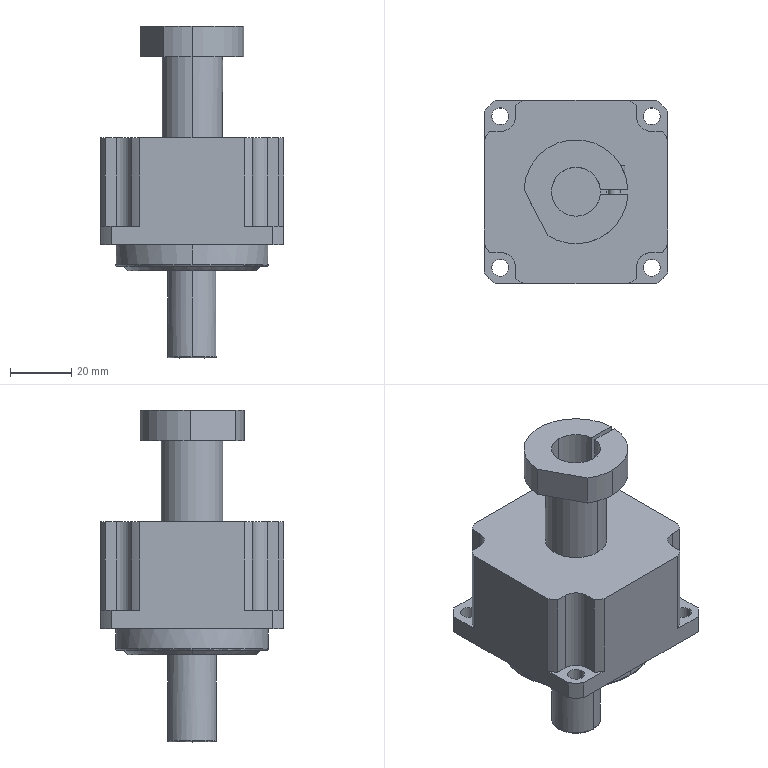Part | NX | 1 solid | 83 faces | box 60 x 60 x 108.5 mm | volume 146086 mm3 | cylinder 42 | plane 29 | cone 6 | torus 6 | commonest cylinder face diameters 5.5 x8 69 x8 10 x4 16 x4 80 x4 34 x3